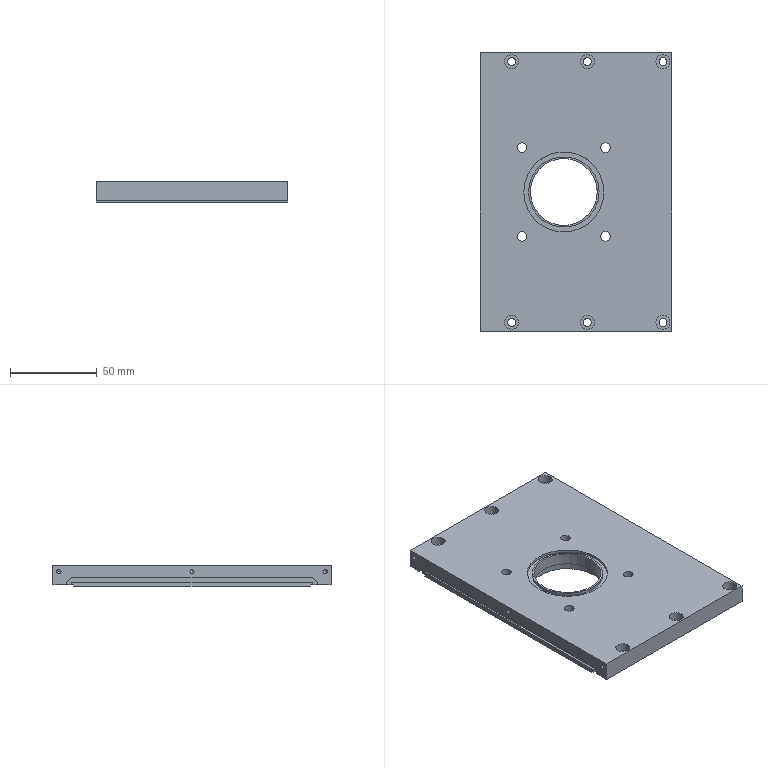NC program | NX | posted with a generic post | part box 110 x 160 x 12 mm
Lines 1 to 30 of 4419:
N10 G17 G21 G94 G90
(DRILLING_COPY_1_COPY , TOOL : D6A45)
N12 T01 M6
N14 G54
N16 G17 G0 G90 X-65. Y0. B0. C0. S5000 M3
N18 G43 Z30. H1
N20 G94 G81 G98 Z-1. F350. R3.
N22 X0.
N24 X45. Y1.
N26 X65. Y0.
N28 G80
N30 G0 X65. Y0. Z30.
N32 M5
(DRILLING_COPY_1_COPY_COPY_COPY_COPY , TOOL : 3.3ZT)
N34 T03 M6
N36 G54
N38 G17 G0 G90 X-65. Y0. B0. C0. S2000 M3
N40 G43 Z30. H3
N42 G94 G83 G98 Z-10.974 F200. Q2. R3.
N44 X0.
N46 X65.
N48 G80
N50 G0 X65. Y0. Z30.
N52 M5